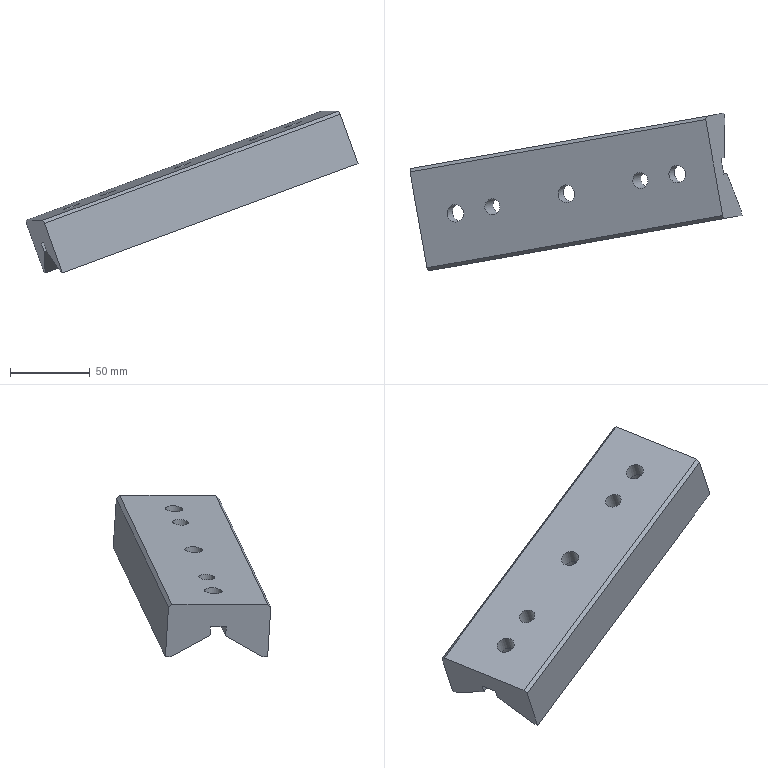Part | NX | features solid 2 | 1 solid | 36 faces | box 207.812 x 98.608 x 101.293 mm | volume 334850 mm3 | plane 28 | cylinder 8 | commonest cylinder face diameters 11 x3 17.5 x3 10 x2
STEP:
#1=CARTESIAN_POINT('',(1039.266,104.665,-184.286));
#2=VERTEX_POINT('',#1);
#3=CARTESIAN_POINT('',(1041.003,94.817,-184.286));
#4=VERTEX_POINT('',#3);
#5=CARTESIAN_POINT('',(1040.138,99.742,-184.285));
#6=DIRECTION('',(-0.3368,-0.05939,0.9397));
#7=DIRECTION('',(-0.9254,-0.1632,-0.342));
#8=AXIS2_PLACEMENT_3D('',#5,#6,#7);
#9=CIRCLE('',#8,5.);
#10=EDGE_CURVE('',#2,#4,#9,.T.);
#11=ORIENTED_EDGE('',*,*,#10,.T.);
#12=CARTESIAN_POINT('',(1001.381,87.831,-198.93));
#13=VERTEX_POINT('',#12);
#14=CARTESIAN_POINT('',(902.194,70.341,-235.588));
#15=DIRECTION('',(0.9254,0.1632,0.342));
#16=VECTOR('',#15,1000.);
#17=LINE('',#14,#16);
#18=EDGE_CURVE('',#13,#4,#17,.T.);
#19=ORIENTED_EDGE('',*,*,#18,.F.);
#20=CARTESIAN_POINT('',(999.644,97.679,-198.93));
#21=VERTEX_POINT('',#20);
#22=CARTESIAN_POINT('',(993.867,91.583,-201.386));
#23=DIRECTION('',(-0.3368,-0.05939,0.9397));
#24=DIRECTION('',(-0.9254,-0.1632,-0.342));
#25=AXIS2_PLACEMENT_3D('',#22,#23,#24);
#26=CIRCLE('',#25,8.75);
#27=EDGE_CURVE('',#13,#21,#26,.T.);
#28=ORIENTED_EDGE('',*,*,#27,.T.);
#29=CARTESIAN_POINT('',(900.458,80.189,-235.588));
#30=DIRECTION('',(0.9254,0.1632,0.342));
#31=VECTOR('',#30,1000.);
#32=LINE('',#29,#31);
#33=EDGE_CURVE('',#21,#2,#32,.T.);
#34=ORIENTED_EDGE('',*,*,#33,.T.);
#35=EDGE_LOOP('',(#11,#19,#28,#34));
#36=FACE_BOUND('',#35,.T.);
#37=CARTESIAN_POINT('',(900.458,80.189,-235.588));
#38=DIRECTION('',(-0.3368,-0.05939,0.9397));
#39=DIRECTION('',(-0.9254,-0.1632,-0.342));
#40=AXIS2_PLACEMENT_3D('',#37,#38,#39);
#41=PLANE('',#40);
#42=ADVANCED_FACE('',(#36),#41,.F.);
#43=CARTESIAN_POINT('',(1039.713,99.667,-168.479));
#44=VERTEX_POINT('',#43);
#45=CARTESIAN_POINT('',(1035.086,98.851,-170.19));
#46=DIRECTION('',(0.3368,0.05939,-0.9397));
#47=DIRECTION('',(0.9254,0.1632,0.342));
#48=AXIS2_PLACEMENT_3D('',#45,#46,#47);
#49=CIRCLE('',#48,5.);
#50=EDGE_CURVE('',#44,#44,#49,.T.);
#51=ORIENTED_EDGE('',*,*,#50,.T.);
#52=EDGE_LOOP('',(#51));
#53=FACE_BOUND('',#52,.T.);
#54=CARTESIAN_POINT('',(983.725,89.795,-189.172));
#55=VERTEX_POINT('',#54);
#56=CARTESIAN_POINT('',(988.815,90.692,-187.291));
#57=DIRECTION('',(0.3368,0.05939,-0.9397));
#58=DIRECTION('',(-0.9254,-0.1632,-0.342));
#59=AXIS2_PLACEMENT_3D('',#56,#57,#58);
#60=CIRCLE('',#59,5.5);
#61=EDGE_CURVE('',#55,#55,#60,.T.);
#62=ORIENTED_EDGE('',*,*,#61,.T.);
#63=EDGE_LOOP('',(#62));
#64=FACE_BOUND('',#63,.T.);
#65=CARTESIAN_POINT('',(947.171,83.349,-202.681));
#66=VERTEX_POINT('',#65);
#67=CARTESIAN_POINT('',(942.544,82.533,-204.392));
#68=DIRECTION('',(0.3368,0.05939,-0.9397));
#69=DIRECTION('',(0.9254,0.1632,0.342));
#70=AXIS2_PLACEMENT_3D('',#67,#68,#69);
#71=CIRCLE('',#70,5.);
#72=EDGE_CURVE('',#66,#66,#71,.T.);
#73=ORIENTED_EDGE('',*,*,#72,.T.);
#74=EDGE_LOOP('',(#73));
#75=FACE_BOUND('',#74,.T.);
#76=CARTESIAN_POINT('',(924.499,79.351,-211.061));
#77=VERTEX_POINT('',#76);
#78=CARTESIAN_POINT('',(919.409,78.454,-212.942));
#79=DIRECTION('',(0.3368,0.05939,-0.9397));
#80=DIRECTION('',(0.9254,0.1632,0.342));
#81=AXIS2_PLACEMENT_3D('',#78,#79,#80);
#82=CIRCLE('',#81,5.5);
#83=EDGE_CURVE('',#77,#77,#82,.T.);
#84=ORIENTED_EDGE('',*,*,#83,.T.);
#85=EDGE_LOOP('',(#84));
#86=FACE_BOUND('',#85,.T.);
#87=CARTESIAN_POINT('',(1063.311,103.828,-159.758));
#88=VERTEX_POINT('',#87);
#89=CARTESIAN_POINT('',(1058.221,102.93,-161.639));
#90=DIRECTION('',(0.3368,0.05939,-0.9397));
#91=DIRECTION('',(0.9254,0.1632,0.342));
#92=AXIS2_PLACEMENT_3D('',#89,#90,#91);
#93=CIRCLE('',#92,5.5);
#94=EDGE_CURVE('',#88,#88,#93,.T.);
#95=ORIENTED_EDGE('',*,*,#94,.T.);
#96=EDGE_LOOP('',(#95));
#97=FACE_BOUND('',#96,.T.);
#98=CARTESIAN_POINT('',(890.977,104.411,-221.493));
#99=VERTEX_POINT('',#98);
#100=CARTESIAN_POINT('',(901.57,44.338,-221.493));
#101=VERTEX_POINT('',#100);
#102=CARTESIAN_POINT('',(890.63,106.381,-221.493));
#103=DIRECTION('',(0.1736,-0.9848,0.));
#104=VECTOR('',#103,1000.);
#105=LINE('',#102,#104);
#106=EDGE_CURVE('',#99,#101,#105,.T.);
#107=ORIENTED_EDGE('',*,*,#106,.T.);
#108=CARTESIAN_POINT('',(1086.653,76.973,-153.089));
#109=VERTEX_POINT('',#108);
#110=CARTESIAN_POINT('',(901.57,44.338,-221.493));
#111=DIRECTION('',(0.9254,0.1632,0.342));
#112=VECTOR('',#111,1000.);
#113=LINE('',#110,#112);
#114=EDGE_CURVE('',#101,#109,#113,.T.);
#115=ORIENTED_EDGE('',*,*,#114,.T.);
#116=CARTESIAN_POINT('',(1076.06,137.046,-153.089));
#117=VERTEX_POINT('',#116);
#118=CARTESIAN_POINT('',(1075.713,139.016,-153.089));
#119=DIRECTION('',(0.1736,-0.9848,0.));
#120=VECTOR('',#119,1000.);
#121=LINE('',#118,#120);
#122=EDGE_CURVE('',#117,#109,#121,.T.);
#123=ORIENTED_EDGE('',*,*,#122,.F.);
#124=CARTESIAN_POINT('',(890.977,104.411,-221.493));
#125=DIRECTION('',(0.9254,0.1632,0.342));
#126=VECTOR('',#125,1000.);
#127=LINE('',#124,#126);
#128=EDGE_CURVE('',#99,#117,#127,.T.);
#129=ORIENTED_EDGE('',*,*,#128,.F.);
#130=EDGE_LOOP('',(#107,#115,#123,#129));
#131=FACE_BOUND('',#130,.T.);
#132=CARTESIAN_POINT('',(890.63,106.381,-221.493));
#133=DIRECTION('',(-0.3368,-0.05939,0.9397));
#134=DIRECTION('',(-0.9254,-0.1632,-0.342));
#135=AXIS2_PLACEMENT_3D('',#132,#133,#134);
#136=PLANE('',#135);
#137=ADVANCED_FACE('',(#53,#64,#75,#86,#97,#131),#136,.T.);
#138=CARTESIAN_POINT('',(946.728,88.348,-218.487));
#139=VERTEX_POINT('',#138);
#140=CARTESIAN_POINT('',(948.465,78.5,-218.487));
#141=VERTEX_POINT('',#140);
#142=CARTESIAN_POINT('',(947.597,83.424,-218.487));
#143=DIRECTION('',(-0.3368,-0.05939,0.9397));
#144=DIRECTION('',(-0.9254,-0.1632,-0.342));
#145=AXIS2_PLACEMENT_3D('',#142,#143,#144);
#146=CIRCLE('',#145,5.);
#147=EDGE_CURVE('',#139,#141,#146,.T.);
#148=ORIENTED_EDGE('',*,*,#147,.T.);
#149=CARTESIAN_POINT('',(931.975,75.592,-224.581));
#150=VERTEX_POINT('',#149);
#151=CARTESIAN_POINT('',(902.194,70.341,-235.588));
#152=DIRECTION('',(0.9254,0.1632,0.342));
#153=VECTOR('',#152,1000.);
#154=LINE('',#151,#153);
#155=EDGE_CURVE('',#150,#141,#154,.T.);
#156=ORIENTED_EDGE('',*,*,#155,.F.);
#157=CARTESIAN_POINT('',(930.238,85.44,-224.581));
#158=VERTEX_POINT('',#157);
#159=CARTESIAN_POINT('',(924.461,79.345,-227.037));
#160=DIRECTION('',(-0.3368,-0.05939,0.9397));
#161=DIRECTION('',(-0.9254,-0.1632,-0.342));
#162=AXIS2_PLACEMENT_3D('',#159,#160,#161);
#163=CIRCLE('',#162,8.75);
#164=EDGE_CURVE('',#150,#158,#163,.T.);
#165=ORIENTED_EDGE('',*,*,#164,.T.);
#166=CARTESIAN_POINT('',(900.458,80.189,-235.588));
#167=DIRECTION('',(0.9254,0.1632,0.342));
#168=VECTOR('',#167,1000.);
#169=LINE('',#166,#168);
#170=EDGE_CURVE('',#158,#139,#169,.T.);
#171=ORIENTED_EDGE('',*,*,#170,.T.);
#172=EDGE_LOOP('',(#148,#156,#165,#171));
#173=FACE_BOUND('',#172,.T.);
#174=CARTESIAN_POINT('',(900.458,80.189,-235.588));
#175=DIRECTION('',(-0.3368,-0.05939,0.9397));
#176=DIRECTION('',(-0.9254,-0.1632,-0.342));
#177=AXIS2_PLACEMENT_3D('',#174,#175,#176);
#178=PLANE('',#177);
#179=ADVANCED_FACE('',(#173),#178,.F.);
#180=CARTESIAN_POINT('',(986.354,95.335,-203.842));
#181=VERTEX_POINT('',#180);
#182=CARTESIAN_POINT('',(988.091,85.487,-203.842));
#183=VERTEX_POINT('',#182);
#184=CARTESIAN_POINT('',(993.867,91.583,-201.386));
#185=DIRECTION('',(-0.3368,-0.05939,0.9397));
#186=DIRECTION('',(-0.9254,-0.1632,-0.342));
#187=AXIS2_PLACEMENT_3D('',#184,#185,#186);
#188=CIRCLE('',#187,8.75);
#189=EDGE_CURVE('',#181,#183,#188,.T.);
#190=ORIENTED_EDGE('',*,*,#189,.T.);
#191=CARTESIAN_POINT('',(902.194,70.341,-235.588));
#192=DIRECTION('',(0.9254,0.1632,0.342));
#193=VECTOR('',#192,1000.);
#194=LINE('',#191,#193);
#195=EDGE_CURVE('',#141,#183,#194,.T.);
#196=ORIENTED_EDGE('',*,*,#195,.F.);
#197=CARTESIAN_POINT('',(947.597,83.424,-218.487));
#198=DIRECTION('',(-0.3368,-0.05939,0.9397));
#199=DIRECTION('',(-0.9254,-0.1632,-0.342));
#200=AXIS2_PLACEMENT_3D('',#197,#198,#199);
#201=CIRCLE('',#200,5.);
#202=EDGE_CURVE('',#141,#139,#201,.T.);
#203=ORIENTED_EDGE('',*,*,#202,.T.);
#204=CARTESIAN_POINT('',(900.458,80.189,-235.588));
#205=DIRECTION('',(0.9254,0.1632,0.342));
#206=VECTOR('',#205,1000.);
#207=LINE('',#204,#206);
#208=EDGE_CURVE('',#139,#181,#207,.T.);
#209=ORIENTED_EDGE('',*,*,#208,.T.);
#210=EDGE_LOOP('',(#190,#196,#203,#209));
#211=FACE_BOUND('',#210,.T.);
#212=CARTESIAN_POINT('',(900.458,80.189,-235.588));
#213=DIRECTION('',(-0.3368,-0.05939,0.9397));
#214=DIRECTION('',(-0.9254,-0.1632,-0.342));
#215=AXIS2_PLACEMENT_3D('',#212,#213,#214);
#216=PLANE('',#215);
#217=ADVANCED_FACE('',(#211),#216,.F.);
#218=CARTESIAN_POINT('',(1055.76,107.573,-178.19));
#219=VERTEX_POINT('',#218);
#220=CARTESIAN_POINT('',(1057.497,97.725,-178.19));
#221=VERTEX_POINT('',#220);
#222=CARTESIAN_POINT('',(1063.274,103.821,-175.734));
#223=DIRECTION('',(-0.3368,-0.05939,0.9397));
#224=DIRECTION('',(-0.9254,-0.1632,-0.342));
#225=AXIS2_PLACEMENT_3D('',#222,#223,#224);
#226=CIRCLE('',#225,8.75);
#227=EDGE_CURVE('',#219,#221,#226,.T.);
#228=ORIENTED_EDGE('',*,*,#227,.T.);
#229=CARTESIAN_POINT('',(902.194,70.341,-235.588));
#230=DIRECTION('',(0.9254,0.1632,0.342));
#231=VECTOR('',#230,1000.);
#232=LINE('',#229,#231);
#233=EDGE_CURVE('',#4,#221,#232,.T.);
#234=ORIENTED_EDGE('',*,*,#233,.F.);
#235=CARTESIAN_POINT('',(1040.138,99.742,-184.285));
#236=DIRECTION('',(-0.3368,-0.05939,0.9397));
#237=DIRECTION('',(-0.9254,-0.1632,-0.342));
#238=AXIS2_PLACEMENT_3D('',#235,#236,#237);
#239=CIRCLE('',#238,5.);
#240=EDGE_CURVE('',#4,#2,#239,.T.);
#241=ORIENTED_EDGE('',*,*,#240,.T.);
#242=CARTESIAN_POINT('',(900.458,80.189,-235.588));
#243=DIRECTION('',(0.9254,0.1632,0.342));
#244=VECTOR('',#243,1000.);
#245=LINE('',#242,#244);
#246=EDGE_CURVE('',#2,#219,#245,.T.);
#247=ORIENTED_EDGE('',*,*,#246,.T.);
#248=EDGE_LOOP('',(#228,#234,#241,#247));
#249=FACE_BOUND('',#248,.T.);
#250=CARTESIAN_POINT('',(900.458,80.189,-235.588));
#251=DIRECTION('',(-0.3368,-0.05939,0.9397));
#252=DIRECTION('',(-0.9254,-0.1632,-0.342));
#253=AXIS2_PLACEMENT_3D('',#250,#251,#252);
#254=PLANE('',#253);
#255=ADVANCED_FACE('',(#249),#254,.F.);
#256=CARTESIAN_POINT('',(1085.541,112.825,-167.184));
#257=VERTEX_POINT('',#256);
#258=CARTESIAN_POINT('',(1087.277,102.976,-167.184));
#259=VERTEX_POINT('',#258);
#260=CARTESIAN_POINT('',(1085.541,112.825,-167.184));
#261=DIRECTION('',(0.1736,-0.9848,0.));
#262=VECTOR('',#261,1000.);
#263=LINE('',#260,#262);
#264=EDGE_CURVE('',#257,#259,#263,.T.);
#265=ORIENTED_EDGE('',*,*,#264,.T.);
#266=CARTESIAN_POINT('',(1070.787,100.069,-173.278));
#267=VERTEX_POINT('',#266);
#268=CARTESIAN_POINT('',(902.194,70.341,-235.588));
#269=DIRECTION('',(0.9254,0.1632,0.342));
#270=VECTOR('',#269,1000.);
#271=LINE('',#268,#270);
#272=EDGE_CURVE('',#267,#259,#271,.T.);
#273=ORIENTED_EDGE('',*,*,#272,.F.);
#274=CARTESIAN_POINT('',(1069.051,109.917,-173.278));
#275=VERTEX_POINT('',#274);
#276=CARTESIAN_POINT('',(1063.274,103.821,-175.734));
#277=DIRECTION('',(-0.3368,-0.05939,0.9397));
#278=DIRECTION('',(-0.9254,-0.1632,-0.342));
#279=AXIS2_PLACEMENT_3D('',#276,#277,#278);
#280=CIRCLE('',#279,8.75);
#281=EDGE_CURVE('',#267,#275,#280,.T.);
#282=ORIENTED_EDGE('',*,*,#281,.T.);
#283=CARTESIAN_POINT('',(900.458,80.189,-235.588));
#284=DIRECTION('',(0.9254,0.1632,0.342));
#285=VECTOR('',#284,1000.);
#286=LINE('',#283,#285);
#287=EDGE_CURVE('',#275,#257,#286,.T.);
#288=ORIENTED_EDGE('',*,*,#287,.T.);
#289=EDGE_LOOP('',(#265,#273,#282,#288));
#290=FACE_BOUND('',#289,.T.);
#291=CARTESIAN_POINT('',(900.458,80.189,-235.588));
#292=DIRECTION('',(-0.3368,-0.05939,0.9397));
#293=DIRECTION('',(-0.9254,-0.1632,-0.342));
#294=AXIS2_PLACEMENT_3D('',#291,#292,#293);
#295=PLANE('',#294);
#296=ADVANCED_FACE('',(#290),#295,.F.);
#297=CARTESIAN_POINT('',(916.948,83.097,-229.493));
#298=VERTEX_POINT('',#297);
#299=CARTESIAN_POINT('',(918.684,73.249,-229.493));
#300=VERTEX_POINT('',#299);
#301=CARTESIAN_POINT('',(924.461,79.345,-227.037));
#302=DIRECTION('',(-0.3368,-0.05939,0.9397));
#303=DIRECTION('',(-0.9254,-0.1632,-0.342));
#304=AXIS2_PLACEMENT_3D('',#301,#302,#303);
#305=CIRCLE('',#304,8.75);
#306=EDGE_CURVE('',#298,#300,#305,.T.);
#307=ORIENTED_EDGE('',*,*,#306,.T.);
#308=CARTESIAN_POINT('',(902.194,70.341,-235.588));
#309=VERTEX_POINT('',#308);
#310=CARTESIAN_POINT('',(902.194,70.341,-235.588));
#311=DIRECTION('',(0.9254,0.1632,0.342));
#312=VECTOR('',#311,1000.);
#313=LINE('',#310,#312);
#314=EDGE_CURVE('',#309,#300,#313,.T.);
#315=ORIENTED_EDGE('',*,*,#314,.F.);
#316=CARTESIAN_POINT('',(900.458,80.189,-235.588));
#317=VERTEX_POINT('',#316);
#318=CARTESIAN_POINT('',(900.458,80.189,-235.588));
#319=DIRECTION('',(0.1736,-0.9848,0.));
#320=VECTOR('',#319,1000.);
#321=LINE('',#318,#320);
#322=EDGE_CURVE('',#317,#309,#321,.T.);
#323=ORIENTED_EDGE('',*,*,#322,.F.);
#324=CARTESIAN_POINT('',(900.458,80.189,-235.588));
#325=DIRECTION('',(0.9254,0.1632,0.342));
#326=VECTOR('',#325,1000.);
#327=LINE('',#324,#326);
#328=EDGE_CURVE('',#317,#298,#327,.T.);
#329=ORIENTED_EDGE('',*,*,#328,.T.);
#330=EDGE_LOOP('',(#307,#315,#323,#329));
#331=FACE_BOUND('',#330,.T.);
#332=CARTESIAN_POINT('',(900.458,80.189,-235.588));
#333=DIRECTION('',(-0.3368,-0.05939,0.9397));
#334=DIRECTION('',(-0.9254,-0.1632,-0.342));
#335=AXIS2_PLACEMENT_3D('',#332,#333,#334);
#336=PLANE('',#335);
#337=ADVANCED_FACE('',(#331),#336,.F.);
#338=ORIENTED_EDGE('',*,*,#322,.T.);
#339=CARTESIAN_POINT('',(904.177,70.691,-241.12));
#340=VERTEX_POINT('',#339);
#341=CARTESIAN_POINT('',(902.194,70.341,-235.588));
#342=DIRECTION('',(0.3368,0.05939,-0.9397));
#343=VECTOR('',#342,1000.);
#344=LINE('',#341,#343);
#345=EDGE_CURVE('',#309,#340,#344,.T.);
#346=ORIENTED_EDGE('',*,*,#345,.T.);
#347=CARTESIAN_POINT('',(913.175,47.456,-254.382));
#348=VERTEX_POINT('',#347);
#349=CARTESIAN_POINT('',(904.177,70.691,-241.12));
#350=DIRECTION('',(0.3188,-0.8232,-0.4698));
#351=VECTOR('',#350,1000.);
#352=LINE('',#349,#351);
#353=EDGE_CURVE('',#340,#348,#352,.T.);
#354=ORIENTED_EDGE('',*,*,#353,.T.);
#355=CARTESIAN_POINT('',(913.706,44.447,-254.382));
#356=VERTEX_POINT('',#355);
#357=CARTESIAN_POINT('',(913.706,44.447,-254.382));
#358=DIRECTION('',(-0.1736,0.9848,0.));
#359=VECTOR('',#358,1000.);
#360=LINE('',#357,#359);
#361=EDGE_CURVE('',#356,#348,#360,.T.);
#362=ORIENTED_EDGE('',*,*,#361,.F.);
#363=CARTESIAN_POINT('',(902.591,42.487,-223.372));
#364=VERTEX_POINT('',#363);
#365=CARTESIAN_POINT('',(901.917,42.368,-221.493));
#366=DIRECTION('',(0.3368,0.05939,-0.9397));
#367=VECTOR('',#366,1000.);
#368=LINE('',#365,#367);
#369=EDGE_CURVE('',#364,#356,#368,.T.);
#370=ORIENTED_EDGE('',*,*,#369,.F.);
#371=CARTESIAN_POINT('',(892.509,60.764,-204.813));
#372=DIRECTION('',(0.361,-0.6544,-0.6645));
#373=VECTOR('',#372,1000.);
#374=LINE('',#371,#373);
#375=EDGE_CURVE('',#364,#101,#374,.F.);
#376=ORIENTED_EDGE('',*,*,#375,.T.);
#377=ORIENTED_EDGE('',*,*,#106,.F.);
#378=CARTESIAN_POINT('',(891.304,106.499,-223.372));
#379=VERTEX_POINT('',#378);
#380=CARTESIAN_POINT('',(888.081,85.877,-204.813));
#381=DIRECTION('',(0.1154,0.7384,-0.6645));
#382=VECTOR('',#381,1000.);
#383=LINE('',#380,#382);
#384=EDGE_CURVE('',#379,#99,#383,.F.);
#385=ORIENTED_EDGE('',*,*,#384,.F.);
#386=CARTESIAN_POINT('',(902.419,108.459,-254.382));
#387=VERTEX_POINT('',#386);
#388=CARTESIAN_POINT('',(890.63,106.381,-221.493));
#389=DIRECTION('',(0.3368,0.05939,-0.9397));
#390=VECTOR('',#389,1000.);
#391=LINE('',#388,#390);
#392=EDGE_CURVE('',#379,#387,#391,.T.);
#393=ORIENTED_EDGE('',*,*,#392,.T.);
#394=CARTESIAN_POINT('',(902.949,105.451,-254.382));
#395=VERTEX_POINT('',#394);
#396=CARTESIAN_POINT('',(902.419,108.459,-254.382));
#397=DIRECTION('',(0.1736,-0.9848,0.));
#398=VECTOR('',#397,1000.);
#399=LINE('',#396,#398);
#400=EDGE_CURVE('',#387,#395,#399,.T.);
#401=ORIENTED_EDGE('',*,*,#400,.T.);
#402=CARTESIAN_POINT('',(902.44,80.539,-241.12));
#403=VERTEX_POINT('',#402);
#404=CARTESIAN_POINT('',(902.44,80.539,-241.12));
#405=DIRECTION('',(0.01803,0.8826,-0.4698));
#406=VECTOR('',#405,1000.);
#407=LINE('',#404,#406);
#408=EDGE_CURVE('',#403,#395,#407,.T.);
#409=ORIENTED_EDGE('',*,*,#408,.F.);
#410=CARTESIAN_POINT('',(900.458,80.189,-235.588));
#411=DIRECTION('',(0.3368,0.05939,-0.9397));
#412=VECTOR('',#411,1000.);
#413=LINE('',#410,#412);
#414=EDGE_CURVE('',#317,#403,#413,.T.);
#415=ORIENTED_EDGE('',*,*,#414,.F.);
#416=EDGE_LOOP('',(#338,#346,#354,#362,#370,#376,#377,#385,#393,#401,#409,#415));
#417=FACE_BOUND('',#416,.T.);
#418=CARTESIAN_POINT('',(895.405,79.298,-221.493));
#419=DIRECTION('',(-0.9254,-0.1632,-0.342));
#420=DIRECTION('',(0.3368,0.05939,-0.9397));
#421=AXIS2_PLACEMENT_3D('',#418,#419,#420);
#422=PLANE('',#421);
#423=ADVANCED_FACE('',(#417),#422,.T.);
#424=ORIENTED_EDGE('',*,*,#122,.T.);
#425=CARTESIAN_POINT('',(1087.674,75.122,-154.968));
#426=VERTEX_POINT('',#425);
#427=CARTESIAN_POINT('',(1086.653,76.973,-153.089));
#428=DIRECTION('',(-0.361,0.6544,0.6645));
#429=VECTOR('',#428,1000.);
#430=LINE('',#427,#429);
#431=EDGE_CURVE('',#109,#426,#430,.F.);
#432=ORIENTED_EDGE('',*,*,#431,.T.);
#433=CARTESIAN_POINT('',(1098.789,77.082,-185.978));
#434=VERTEX_POINT('',#433);
#435=CARTESIAN_POINT('',(1087.,75.003,-153.089));
#436=DIRECTION('',(0.3368,0.05939,-0.9397));
#437=VECTOR('',#436,1000.);
#438=LINE('',#435,#437);
#439=EDGE_CURVE('',#426,#434,#438,.T.);
#440=ORIENTED_EDGE('',*,*,#439,.T.);
#441=CARTESIAN_POINT('',(1098.259,80.091,-185.978));
#442=VERTEX_POINT('',#441);
#443=CARTESIAN_POINT('',(1098.789,77.082,-185.978));
#444=DIRECTION('',(-0.1736,0.9848,0.));
#445=VECTOR('',#444,1000.);
#446=LINE('',#443,#445);
#447=EDGE_CURVE('',#434,#442,#446,.T.);
#448=ORIENTED_EDGE('',*,*,#447,.T.);
#449=CARTESIAN_POINT('',(1089.26,103.326,-172.716));
#450=VERTEX_POINT('',#449);
#451=CARTESIAN_POINT('',(1089.26,103.326,-172.716));
#452=DIRECTION('',(0.3188,-0.8232,-0.4698));
#453=VECTOR('',#452,1000.);
#454=LINE('',#451,#453);
#455=EDGE_CURVE('',#450,#442,#454,.T.);
#456=ORIENTED_EDGE('',*,*,#455,.F.);
#457=CARTESIAN_POINT('',(1087.277,102.976,-167.184));
#458=DIRECTION('',(0.3368,0.05939,-0.9397));
#459=VECTOR('',#458,1000.);
#460=LINE('',#457,#459);
#461=EDGE_CURVE('',#259,#450,#460,.T.);
#462=ORIENTED_EDGE('',*,*,#461,.F.);
#463=ORIENTED_EDGE('',*,*,#264,.F.);
#464=CARTESIAN_POINT('',(1087.524,113.174,-172.716));
#465=VERTEX_POINT('',#464);
#466=CARTESIAN_POINT('',(1085.541,112.825,-167.184));
#467=DIRECTION('',(0.3368,0.05939,-0.9397));
#468=VECTOR('',#467,1000.);
#469=LINE('',#466,#468);
#470=EDGE_CURVE('',#257,#465,#469,.T.);
#471=ORIENTED_EDGE('',*,*,#470,.T.);
#472=CARTESIAN_POINT('',(1088.033,138.086,-185.978));
#473=VERTEX_POINT('',#472);
#474=CARTESIAN_POINT('',(1087.524,113.174,-172.716));
#475=DIRECTION('',(0.01803,0.8826,-0.4698));
#476=VECTOR('',#475,1000.);
#477=LINE('',#474,#476);
#478=EDGE_CURVE('',#465,#473,#477,.T.);
#479=ORIENTED_EDGE('',*,*,#478,.T.);
#480=CARTESIAN_POINT('',(1087.502,141.095,-185.978));
#481=VERTEX_POINT('',#480);
#482=CARTESIAN_POINT('',(1087.502,141.095,-185.978));
#483=DIRECTION('',(0.1736,-0.9848,0.));
#484=VECTOR('',#483,1000.);
#485=LINE('',#482,#484);
#486=EDGE_CURVE('',#481,#473,#485,.T.);
#487=ORIENTED_EDGE('',*,*,#486,.F.);
#488=CARTESIAN_POINT('',(1076.387,139.135,-154.968));
#489=VERTEX_POINT('',#488);
#490=CARTESIAN_POINT('',(1075.713,139.016,-153.089));
#491=DIRECTION('',(0.3368,0.05939,-0.9397));
#492=VECTOR('',#491,1000.);
#493=LINE('',#490,#492);
#494=EDGE_CURVE('',#489,#481,#493,.T.);
#495=ORIENTED_EDGE('',*,*,#494,.F.);
#496=CARTESIAN_POINT('',(1076.06,137.046,-153.089));
#497=DIRECTION('',(-0.1154,-0.7384,0.6645));
#498=VECTOR('',#497,1000.);
#499=LINE('',#496,#498);
#500=EDGE_CURVE('',#117,#489,#499,.F.);
#501=ORIENTED_EDGE('',*,*,#500,.F.);
#502=EDGE_LOOP('',(#424,#432,#440,#448,#456,#462,#463,#471,#479,#487,#495,#501));
#503=FACE_BOUND('',#502,.T.);
#504=CARTESIAN_POINT('',(1080.489,111.934,-153.089));
#505=DIRECTION('',(-0.9254,-0.1632,-0.342));
#506=DIRECTION('',(0.3368,0.05939,-0.9397));
#507=AXIS2_PLACEMENT_3D('',#504,#505,#506);
#508=PLANE('',#507);
#509=ADVANCED_FACE('',(#503),#508,.F.);
#510=ORIENTED_EDGE('',*,*,#94,.F.);
#511=EDGE_LOOP('',(#510));
#512=FACE_BOUND('',#511,.T.);
#513=CARTESIAN_POINT('',(1066.767,103.524,-169.18));
#514=VERTEX_POINT('',#513);
#515=CARTESIAN_POINT('',(1061.59,103.524,-171.036));
#516=DIRECTION('',(-0.3368,-0.05939,0.9397));
#517=DIRECTION('',(0.9414,0.,0.3374));
#518=AXIS2_PLACEMENT_3D('',#515,#516,#517);
#519=CIRCLE('',#518,5.5);
#520=EDGE_CURVE('',#514,#514,#519,.F.);
#521=ORIENTED_EDGE('',*,*,#520,.T.);
#522=EDGE_LOOP('',(#521));
#523=FACE_BOUND('',#522,.T.);
#524=CARTESIAN_POINT('',(1058.221,102.93,-161.639));
#525=DIRECTION('',(0.3368,0.05939,-0.9397));
#526=DIRECTION('',(0.9254,0.1632,0.342));
#527=AXIS2_PLACEMENT_3D('',#524,#525,#526);
#528=CYLINDRICAL_SURFACE('',#527,5.5);
#529=ADVANCED_FACE('',(#512,#523),#528,.F.);
#530=CARTESIAN_POINT('',(1069.826,103.524,-168.084));
#531=VERTEX_POINT('',#530);
#532=CARTESIAN_POINT('',(1061.59,103.524,-171.036));
#533=DIRECTION('',(-0.3368,-0.05939,0.9397));
#534=DIRECTION('',(0.9414,0.,0.3374));
#535=AXIS2_PLACEMENT_3D('',#532,#533,#534);
#536=CIRCLE('',#535,8.75);
#537=EDGE_CURVE('',#531,#531,#536,.F.);
#538=ORIENTED_EDGE('',*,*,#537,.F.);
#539=EDGE_LOOP('',(#538));
#540=FACE_BOUND('',#539,.T.);
#541=CARTESIAN_POINT('',(1059.48,98.075,-183.722));
#542=VERTEX_POINT('',#541);
#543=CARTESIAN_POINT('',(1055.139,97.31,-171.612));
#544=DIRECTION('',(0.3368,0.05939,-0.9397));
#545=VECTOR('',#544,1000.);
#546=LINE('',#543,#545);
#547=EDGE_CURVE('',#221,#542,#546,.T.);
#548=ORIENTED_EDGE('',*,*,#547,.F.);
#549=ORIENTED_EDGE('',*,*,#227,.F.);
#550=CARTESIAN_POINT('',(1057.743,107.923,-183.722));
#551=VERTEX_POINT('',#550);
#552=CARTESIAN_POINT('',(1053.403,107.158,-171.612));
#553=DIRECTION('',(0.3368,0.05939,-0.9397));
#554=VECTOR('',#553,1000.);
#555=LINE('',#552,#554);
#556=EDGE_CURVE('',#219,#551,#555,.T.);
#557=ORIENTED_EDGE('',*,*,#556,.T.);
#558=CARTESIAN_POINT('',(1071.033,110.266,-178.81));
#559=VERTEX_POINT('',#558);
#560=CARTESIAN_POINT('',(1064.284,103.999,-178.553));
#561=DIRECTION('',(0.3785,-0.441,-0.8138));
#562=DIRECTION('',(0.01803,0.8826,-0.4698));
#563=AXIS2_PLACEMENT_3D('',#560,#561,#562);
#564=ELLIPSE('',#563,10.104,8.75);
#565=EDGE_CURVE('',#551,#559,#564,.T.);
#566=ORIENTED_EDGE('',*,*,#565,.T.);
#567=CARTESIAN_POINT('',(1066.693,109.501,-166.701));
#568=DIRECTION('',(0.3368,0.05939,-0.9397));
#569=VECTOR('',#568,1000.);
#570=LINE('',#567,#569);
#571=EDGE_CURVE('',#559,#275,#570,.F.);
#572=ORIENTED_EDGE('',*,*,#571,.T.);
#573=ORIENTED_EDGE('',*,*,#281,.F.);
#574=CARTESIAN_POINT('',(1072.77,100.418,-178.81));
#575=VERTEX_POINT('',#574);
#576=CARTESIAN_POINT('',(1068.429,99.653,-166.701));
#577=DIRECTION('',(0.3368,0.05939,-0.9397));
#578=VECTOR('',#577,1000.);
#579=LINE('',#576,#578);
#580=EDGE_CURVE('',#575,#267,#579,.F.);
#581=ORIENTED_EDGE('',*,*,#580,.F.);
#582=CARTESIAN_POINT('',(1064.284,103.999,-178.553));
#583=DIRECTION('',(-0.2049,-0.5438,0.8138));
#584=DIRECTION('',(0.3188,-0.8232,-0.4698));
#585=AXIS2_PLACEMENT_3D('',#582,#583,#584);
#586=ELLIPSE('',#585,10.104,8.75);
#587=EDGE_CURVE('',#542,#575,#586,.T.);
#588=ORIENTED_EDGE('',*,*,#587,.F.);
#589=EDGE_LOOP('',(#548,#549,#557,#566,#572,#573,#581,#588));
#590=FACE_BOUND('',#589,.T.);
#591=CARTESIAN_POINT('',(1060.916,103.405,-169.157));
#592=DIRECTION('',(0.3368,0.05939,-0.9397));
#593=DIRECTION('',(0.9254,0.1632,0.342));
#594=AXIS2_PLACEMENT_3D('',#591,#592,#593);
#595=CYLINDRICAL_SURFACE('',#594,8.75);
#596=ADVANCED_FACE('',(#540,#590),#595,.F.);
#597=ORIENTED_EDGE('',*,*,#520,.F.);
#598=EDGE_LOOP('',(#597));
#599=FACE_BOUND('',#598,.T.);
#600=ORIENTED_EDGE('',*,*,#537,.T.);
#601=EDGE_LOOP('',(#600));
#602=FACE_BOUND('',#601,.T.);
#603=CARTESIAN_POINT('',(1015.319,95.365,-188.137));
#604=DIRECTION('',(-0.3368,-0.05939,0.9397));
#605=DIRECTION('',(-0.9254,-0.1632,-0.342));
#606=AXIS2_PLACEMENT_3D('',#603,#604,#605);
#607=PLANE('',#606);
#608=ADVANCED_FACE('',(#599,#602),#607,.F.);
#609=ORIENTED_EDGE('',*,*,#50,.F.);
#610=EDGE_LOOP('',(#609));
#611=FACE_BOUND('',#610,.T.);
#612=ORIENTED_EDGE('',*,*,#240,.F.);
#613=ORIENTED_EDGE('',*,*,#10,.F.);
#614=EDGE_LOOP('',(#612,#613));
#615=FACE_BOUND('',#614,.T.);
#616=CARTESIAN_POINT('',(1035.086,98.851,-170.19));
#617=DIRECTION('',(0.3368,0.05939,-0.9397));
#618=DIRECTION('',(0.9254,0.1632,0.342));
#619=AXIS2_PLACEMENT_3D('',#616,#617,#618);
#620=CYLINDRICAL_SURFACE('',#619,5.);
#621=ADVANCED_FACE('',(#611,#615),#620,.F.);
#622=ORIENTED_EDGE('',*,*,#72,.F.);
#623=EDGE_LOOP('',(#622));
#624=FACE_BOUND('',#623,.T.);
#625=ORIENTED_EDGE('',*,*,#202,.F.);
#626=ORIENTED_EDGE('',*,*,#147,.F.);
#627=EDGE_LOOP('',(#625,#626));
#628=FACE_BOUND('',#627,.T.);
#629=CARTESIAN_POINT('',(942.544,82.533,-204.392));
#630=DIRECTION('',(0.3368,0.05939,-0.9397));
#631=DIRECTION('',(0.9254,0.1632,0.342));
#632=AXIS2_PLACEMENT_3D('',#629,#630,#631);
#633=CYLINDRICAL_SURFACE('',#632,5.);
#634=ADVANCED_FACE('',(#624,#628),#633,.F.);
#635=CARTESIAN_POINT('',(927.955,79.048,-220.483));
#636=VERTEX_POINT('',#635);
#637=CARTESIAN_POINT('',(922.777,79.048,-222.339));
#638=DIRECTION('',(-0.3368,-0.05939,0.9397));
#639=DIRECTION('',(0.9414,0.,0.3374));
#640=AXIS2_PLACEMENT_3D('',#637,#638,#639);
#641=CIRCLE('',#640,5.5);
#642=EDGE_CURVE('',#636,#636,#641,.F.);
#643=ORIENTED_EDGE('',*,*,#642,.T.);
#644=EDGE_LOOP('',(#643));
#645=FACE_BOUND('',#644,.T.);
#646=ORIENTED_EDGE('',*,*,#83,.F.);
#647=EDGE_LOOP('',(#646));
#648=FACE_BOUND('',#647,.T.);
#649=CARTESIAN_POINT('',(919.409,78.454,-212.942));
#650=DIRECTION('',(0.3368,0.05939,-0.9397));
#651=DIRECTION('',(0.9254,0.1632,0.342));
#652=AXIS2_PLACEMENT_3D('',#649,#650,#651);
#653=CYLINDRICAL_SURFACE('',#652,5.5);
#654=ADVANCED_FACE('',(#645,#648),#653,.F.);
#655=ORIENTED_EDGE('',*,*,#164,.F.);
#656=CARTESIAN_POINT('',(933.957,75.942,-230.113));
#657=VERTEX_POINT('',#656);
#658=CARTESIAN_POINT('',(929.617,75.177,-218.004));
#659=DIRECTION('',(0.3368,0.05939,-0.9397));
#660=VECTOR('',#659,1000.);
#661=LINE('',#658,#660);
#662=EDGE_CURVE('',#657,#150,#661,.F.);
#663=ORIENTED_EDGE('',*,*,#662,.F.);
#664=CARTESIAN_POINT('',(920.667,73.599,-235.025));
#665=VERTEX_POINT('',#664);
#666=CARTESIAN_POINT('',(925.472,79.523,-229.856));
#667=DIRECTION('',(-0.2049,-0.5438,0.8138));
#668=DIRECTION('',(0.3188,-0.8232,-0.4698));
#669=AXIS2_PLACEMENT_3D('',#666,#667,#668);
#670=ELLIPSE('',#669,10.104,8.75);
#671=EDGE_CURVE('',#665,#657,#670,.T.);
#672=ORIENTED_EDGE('',*,*,#671,.F.);
#673=CARTESIAN_POINT('',(916.327,72.833,-222.916));
#674=DIRECTION('',(0.3368,0.05939,-0.9397));
#675=VECTOR('',#674,1000.);
#676=LINE('',#673,#675);
#677=EDGE_CURVE('',#300,#665,#676,.T.);
#678=ORIENTED_EDGE('',*,*,#677,.F.);
#679=ORIENTED_EDGE('',*,*,#306,.F.);
#680=CARTESIAN_POINT('',(918.931,83.447,-235.025));
#681=VERTEX_POINT('',#680);
#682=CARTESIAN_POINT('',(914.59,82.681,-222.916));
#683=DIRECTION('',(0.3368,0.05939,-0.9397));
#684=VECTOR('',#683,1000.);
#685=LINE('',#682,#684);
#686=EDGE_CURVE('',#298,#681,#685,.T.);
#687=ORIENTED_EDGE('',*,*,#686,.T.);
#688=CARTESIAN_POINT('',(932.221,85.79,-230.113));
#689=VERTEX_POINT('',#688);
#690=CARTESIAN_POINT('',(925.472,79.523,-229.856));
#691=DIRECTION('',(0.3785,-0.441,-0.8138));
#692=DIRECTION('',(0.01803,0.8826,-0.4698));
#693=AXIS2_PLACEMENT_3D('',#690,#691,#692);
#694=ELLIPSE('',#693,10.104,8.75);
#695=EDGE_CURVE('',#681,#689,#694,.T.);
#696=ORIENTED_EDGE('',*,*,#695,.T.);
#697=CARTESIAN_POINT('',(927.88,85.025,-218.004));
#698=DIRECTION('',(0.3368,0.05939,-0.9397));
#699=VECTOR('',#698,1000.);
#700=LINE('',#697,#699);
#701=EDGE_CURVE('',#689,#158,#700,.F.);
#702=ORIENTED_EDGE('',*,*,#701,.T.);
#703=EDGE_LOOP('',(#655,#663,#672,#678,#679,#687,#696,#702));
#704=FACE_BOUND('',#703,.T.);
#705=CARTESIAN_POINT('',(931.014,79.048,-219.387));
#706=VERTEX_POINT('',#705);
#707=CARTESIAN_POINT('',(922.777,79.048,-222.339));
#708=DIRECTION('',(-0.3368,-0.05939,0.9397));
#709=DIRECTION('',(0.9414,0.,0.3374));
#710=AXIS2_PLACEMENT_3D('',#707,#708,#709);
#711=CIRCLE('',#710,8.75);
#712=EDGE_CURVE('',#706,#706,#711,.F.);
#713=ORIENTED_EDGE('',*,*,#712,.F.);
#714=EDGE_LOOP('',(#713));
#715=FACE_BOUND('',#714,.T.);
#716=CARTESIAN_POINT('',(922.103,78.929,-220.46));
#717=DIRECTION('',(0.3368,0.05939,-0.9397));
#718=DIRECTION('',(0.9254,0.1632,0.342));
#719=AXIS2_PLACEMENT_3D('',#716,#717,#718);
#720=CYLINDRICAL_SURFACE('',#719,8.75);
#721=ADVANCED_FACE('',(#704,#715),#720,.F.);
#722=ORIENTED_EDGE('',*,*,#712,.T.);
#723=EDGE_LOOP('',(#722));
#724=FACE_BOUND('',#723,.T.);
#725=ORIENTED_EDGE('',*,*,#642,.F.);
#726=EDGE_LOOP('',(#725));
#727=FACE_BOUND('',#726,.T.);
#728=CARTESIAN_POINT('',(922.777,79.048,-222.339));
#729=DIRECTION('',(-0.3368,-0.05939,0.9397));
#730=DIRECTION('',(-0.9254,-0.1632,-0.342));
#731=AXIS2_PLACEMENT_3D('',#728,#729,#730);
#732=PLANE('',#731);
#733=ADVANCED_FACE('',(#724,#727),#732,.F.);
#734=ORIENTED_EDGE('',*,*,#27,.F.);
#735=CARTESIAN_POINT('',(1003.364,88.18,-204.462));
#736=VERTEX_POINT('',#735);
#737=CARTESIAN_POINT('',(999.023,87.415,-192.352));
#738=DIRECTION('',(0.3368,0.05939,-0.9397));
#739=VECTOR('',#738,1000.);
#740=LINE('',#737,#739);
#741=EDGE_CURVE('',#13,#736,#740,.T.);
#742=ORIENTED_EDGE('',*,*,#741,.T.);
#743=CARTESIAN_POINT('',(990.073,85.837,-209.374));
#744=VERTEX_POINT('',#743);
#745=CARTESIAN_POINT('',(994.878,91.761,-204.205));
#746=DIRECTION('',(0.2049,0.5438,-0.8138));
#747=DIRECTION('',(0.3188,-0.8232,-0.4698));
#748=AXIS2_PLACEMENT_3D('',#745,#746,#747);
#749=ELLIPSE('',#748,10.104,8.75);
#750=EDGE_CURVE('',#736,#744,#749,.T.);
#751=ORIENTED_EDGE('',*,*,#750,.T.);
#752=CARTESIAN_POINT('',(985.733,85.071,-197.264));
#753=DIRECTION('',(0.3368,0.05939,-0.9397));
#754=VECTOR('',#753,1000.);
#755=LINE('',#752,#754);
#756=EDGE_CURVE('',#744,#183,#755,.F.);
#757=ORIENTED_EDGE('',*,*,#756,.T.);
#758=ORIENTED_EDGE('',*,*,#189,.F.);
#759=CARTESIAN_POINT('',(988.337,95.685,-209.374));
#760=VERTEX_POINT('',#759);
#761=CARTESIAN_POINT('',(983.996,94.919,-197.264));
#762=DIRECTION('',(0.3368,0.05939,-0.9397));
#763=VECTOR('',#762,1000.);
#764=LINE('',#761,#763);
#765=EDGE_CURVE('',#760,#181,#764,.F.);
#766=ORIENTED_EDGE('',*,*,#765,.F.);
#767=CARTESIAN_POINT('',(1001.627,98.028,-204.462));
#768=VERTEX_POINT('',#767);
#769=CARTESIAN_POINT('',(994.878,91.761,-204.205));
#770=DIRECTION('',(-0.3785,0.441,0.8138));
#771=DIRECTION('',(0.01803,0.8826,-0.4698));
#772=AXIS2_PLACEMENT_3D('',#769,#770,#771);
#773=ELLIPSE('',#772,10.104,8.75);
#774=EDGE_CURVE('',#768,#760,#773,.T.);
#775=ORIENTED_EDGE('',*,*,#774,.F.);
#776=CARTESIAN_POINT('',(997.287,97.263,-192.352));
#777=DIRECTION('',(0.3368,0.05939,-0.9397));
#778=VECTOR('',#777,1000.);
#779=LINE('',#776,#778);
#780=EDGE_CURVE('',#21,#768,#779,.T.);
#781=ORIENTED_EDGE('',*,*,#780,.F.);
#782=EDGE_LOOP('',(#734,#742,#751,#757,#758,#766,#775,#781));
#783=FACE_BOUND('',#782,.T.);
#784=CARTESIAN_POINT('',(1000.42,91.286,-193.735));
#785=VERTEX_POINT('',#784);
#786=CARTESIAN_POINT('',(992.183,91.286,-196.687));
#787=DIRECTION('',(-0.3368,-0.05939,0.9397));
#788=DIRECTION('',(0.9414,0.,0.3374));
#789=AXIS2_PLACEMENT_3D('',#786,#787,#788);
#790=CIRCLE('',#789,8.75);
#791=EDGE_CURVE('',#785,#785,#790,.T.);
#792=ORIENTED_EDGE('',*,*,#791,.T.);
#793=EDGE_LOOP('',(#792));
#794=FACE_BOUND('',#793,.T.);
#795=CARTESIAN_POINT('',(991.51,91.167,-194.808));
#796=DIRECTION('',(0.3368,0.05939,-0.9397));
#797=DIRECTION('',(-0.9254,-0.1632,-0.342));
#798=AXIS2_PLACEMENT_3D('',#795,#796,#797);
#799=CYLINDRICAL_SURFACE('',#798,8.75);
#800=ADVANCED_FACE('',(#783,#794),#799,.F.);
#801=ORIENTED_EDGE('',*,*,#791,.F.);
#802=EDGE_LOOP('',(#801));
#803=FACE_BOUND('',#802,.T.);
#804=CARTESIAN_POINT('',(997.361,91.286,-194.832));
#805=VERTEX_POINT('',#804);
#806=CARTESIAN_POINT('',(992.183,91.286,-196.687));
#807=DIRECTION('',(-0.3368,-0.05939,0.9397));
#808=DIRECTION('',(0.9414,0.,0.3374));
#809=AXIS2_PLACEMENT_3D('',#806,#807,#808);
#810=CIRCLE('',#809,5.5);
#811=EDGE_CURVE('',#805,#805,#810,.T.);
#812=ORIENTED_EDGE('',*,*,#811,.T.);
#813=EDGE_LOOP('',(#812));
#814=FACE_BOUND('',#813,.T.);
#815=CARTESIAN_POINT('',(992.183,91.286,-196.687));
#816=DIRECTION('',(-0.3368,-0.05939,0.9397));
#817=DIRECTION('',(0.9254,0.1632,0.342));
#818=AXIS2_PLACEMENT_3D('',#815,#816,#817);
#819=PLANE('',#818);
#820=ADVANCED_FACE('',(#803,#814),#819,.F.);
#821=ORIENTED_EDGE('',*,*,#61,.F.);
#822=EDGE_LOOP('',(#821));
#823=FACE_BOUND('',#822,.T.);
#824=ORIENTED_EDGE('',*,*,#811,.F.);
#825=EDGE_LOOP('',(#824));
#826=FACE_BOUND('',#825,.T.);
#827=CARTESIAN_POINT('',(988.815,90.692,-187.291));
#828=DIRECTION('',(0.3368,0.05939,-0.9397));
#829=DIRECTION('',(-0.9254,-0.1632,-0.342));
#830=AXIS2_PLACEMENT_3D('',#827,#828,#829);
#831=CYLINDRICAL_SURFACE('',#830,5.5);
#832=ADVANCED_FACE('',(#823,#826),#831,.F.);
#833=ORIENTED_EDGE('',*,*,#33,.F.);
#834=ORIENTED_EDGE('',*,*,#780,.T.);
#835=CARTESIAN_POINT('',(902.44,80.539,-241.12));
#836=DIRECTION('',(0.9254,0.1632,0.342));
#837=VECTOR('',#836,1000.);
#838=LINE('',#835,#837);
#839=EDGE_CURVE('',#768,#551,#838,.T.);
#840=ORIENTED_EDGE('',*,*,#839,.T.);
#841=ORIENTED_EDGE('',*,*,#556,.F.);
#842=ORIENTED_EDGE('',*,*,#246,.F.);
#843=EDGE_LOOP('',(#833,#834,#840,#841,#842));
#844=FACE_BOUND('',#843,.T.);
#845=CARTESIAN_POINT('',(900.458,80.189,-235.588));
#846=DIRECTION('',(-0.1736,0.9848,0.));
#847=DIRECTION('',(-0.3368,-0.05939,0.9397));
#848=AXIS2_PLACEMENT_3D('',#845,#846,#847);
#849=PLANE('',#848);
#850=ADVANCED_FACE('',(#844),#849,.F.);
#851=ORIENTED_EDGE('',*,*,#328,.F.);
#852=ORIENTED_EDGE('',*,*,#414,.T.);
#853=CARTESIAN_POINT('',(902.44,80.539,-241.12));
#854=DIRECTION('',(0.9254,0.1632,0.342));
#855=VECTOR('',#854,1000.);
#856=LINE('',#853,#855);
#857=EDGE_CURVE('',#403,#681,#856,.T.);
#858=ORIENTED_EDGE('',*,*,#857,.T.);
#859=ORIENTED_EDGE('',*,*,#686,.F.);
#860=EDGE_LOOP('',(#851,#852,#858,#859));
#861=FACE_BOUND('',#860,.T.);
#862=CARTESIAN_POINT('',(900.458,80.189,-235.588));
#863=DIRECTION('',(-0.1736,0.9848,0.));
#864=DIRECTION('',(-0.3368,-0.05939,0.9397));
#865=AXIS2_PLACEMENT_3D('',#862,#863,#864);
#866=PLANE('',#865);
#867=ADVANCED_FACE('',(#861),#866,.F.);
#868=ORIENTED_EDGE('',*,*,#701,.F.);
#869=CARTESIAN_POINT('',(902.44,80.539,-241.12));
#870=DIRECTION('',(-0.9254,-0.1632,-0.342));
#871=VECTOR('',#870,1000.);
#872=LINE('',#869,#871);
#873=EDGE_CURVE('',#689,#760,#872,.F.);
#874=ORIENTED_EDGE('',*,*,#873,.T.);
#875=ORIENTED_EDGE('',*,*,#765,.T.);
#876=ORIENTED_EDGE('',*,*,#208,.F.);
#877=ORIENTED_EDGE('',*,*,#170,.F.);
#878=EDGE_LOOP('',(#868,#874,#875,#876,#877));
#879=FACE_BOUND('',#878,.T.);
#880=CARTESIAN_POINT('',(900.458,80.189,-235.588));
#881=DIRECTION('',(-0.1736,0.9848,0.));
#882=DIRECTION('',(-0.3368,-0.05939,0.9397));
#883=AXIS2_PLACEMENT_3D('',#880,#881,#882);
#884=PLANE('',#883);
#885=ADVANCED_FACE('',(#879),#884,.F.);
#886=ORIENTED_EDGE('',*,*,#494,.T.);
#887=CARTESIAN_POINT('',(902.419,108.459,-254.382));
#888=DIRECTION('',(0.9254,0.1632,0.342));
#889=VECTOR('',#888,1000.);
#890=LINE('',#887,#889);
#891=EDGE_CURVE('',#387,#481,#890,.T.);
#892=ORIENTED_EDGE('',*,*,#891,.F.);
#893=ORIENTED_EDGE('',*,*,#392,.F.);
#894=CARTESIAN_POINT('',(891.304,106.499,-223.372));
#895=DIRECTION('',(-0.9254,-0.1632,-0.342));
#896=VECTOR('',#895,1000.);
#897=LINE('',#894,#896);
#898=EDGE_CURVE('',#489,#379,#897,.T.);
#899=ORIENTED_EDGE('',*,*,#898,.F.);
#900=EDGE_LOOP('',(#886,#892,#893,#899));
#901=FACE_BOUND('',#900,.T.);
#902=CARTESIAN_POINT('',(890.63,106.381,-221.493));
#903=DIRECTION('',(-0.1736,0.9848,0.));
#904=DIRECTION('',(-0.3368,-0.05939,0.9397));
#905=AXIS2_PLACEMENT_3D('',#902,#903,#904);
#906=PLANE('',#905);
#907=ADVANCED_FACE('',(#901),#906,.T.);
#908=ORIENTED_EDGE('',*,*,#486,.T.);
#909=CARTESIAN_POINT('',(902.949,105.451,-254.382));
#910=DIRECTION('',(0.9254,0.1632,0.342));
#911=VECTOR('',#910,1000.);
#912=LINE('',#909,#911);
#913=EDGE_CURVE('',#395,#473,#912,.T.);
#914=ORIENTED_EDGE('',*,*,#913,.F.);
#915=ORIENTED_EDGE('',*,*,#400,.F.);
#916=ORIENTED_EDGE('',*,*,#891,.T.);
#917=EDGE_LOOP('',(#908,#914,#915,#916));
#918=FACE_BOUND('',#917,.T.);
#919=CARTESIAN_POINT('',(902.419,108.459,-254.382));
#920=DIRECTION('',(0.3368,0.05939,-0.9397));
#921=DIRECTION('',(0.9254,0.1632,0.342));
#922=AXIS2_PLACEMENT_3D('',#919,#920,#921);
#923=PLANE('',#922);
#924=ADVANCED_FACE('',(#918),#923,.T.);
#925=ORIENTED_EDGE('',*,*,#839,.F.);
#926=ORIENTED_EDGE('',*,*,#774,.T.);
#927=ORIENTED_EDGE('',*,*,#873,.F.);
#928=ORIENTED_EDGE('',*,*,#695,.F.);
#929=ORIENTED_EDGE('',*,*,#857,.F.);
#930=ORIENTED_EDGE('',*,*,#408,.T.);
#931=ORIENTED_EDGE('',*,*,#913,.T.);
#932=ORIENTED_EDGE('',*,*,#478,.F.);
#933=CARTESIAN_POINT('',(902.44,80.539,-241.12));
#934=DIRECTION('',(0.9254,0.1632,0.342));
#935=VECTOR('',#934,1000.);
#936=LINE('',#933,#935);
#937=EDGE_CURVE('',#559,#465,#936,.T.);
#938=ORIENTED_EDGE('',*,*,#937,.F.);
#939=ORIENTED_EDGE('',*,*,#565,.F.);
#940=EDGE_LOOP('',(#925,#926,#927,#928,#929,#930,#931,#932,#938,#939));
#941=FACE_BOUND('',#940,.T.);
#942=CARTESIAN_POINT('',(902.44,80.539,-241.12));
#943=DIRECTION('',(-0.3785,0.441,0.8138));
#944=DIRECTION('',(-0.01803,-0.8826,0.4698));
#945=AXIS2_PLACEMENT_3D('',#942,#943,#944);
#946=PLANE('',#945);
#947=ADVANCED_FACE('',(#941),#946,.F.);
#948=ORIENTED_EDGE('',*,*,#937,.T.);
#949=ORIENTED_EDGE('',*,*,#470,.F.);
#950=ORIENTED_EDGE('',*,*,#287,.F.);
#951=ORIENTED_EDGE('',*,*,#571,.F.);
#952=EDGE_LOOP('',(#948,#949,#950,#951));
#953=FACE_BOUND('',#952,.T.);
#954=CARTESIAN_POINT('',(900.458,80.189,-235.588));
#955=DIRECTION('',(-0.1736,0.9848,0.));
#956=DIRECTION('',(-0.3368,-0.05939,0.9397));
#957=AXIS2_PLACEMENT_3D('',#954,#955,#956);
#958=PLANE('',#957);
#959=ADVANCED_FACE('',(#953),#958,.F.);
#960=ORIENTED_EDGE('',*,*,#384,.T.);
#961=ORIENTED_EDGE('',*,*,#128,.T.);
#962=ORIENTED_EDGE('',*,*,#500,.T.);
#963=ORIENTED_EDGE('',*,*,#898,.T.);
#964=EDGE_LOOP('',(#960,#961,#962,#963));
#965=FACE_BOUND('',#964,.T.);
#966=CARTESIAN_POINT('',(890.977,104.411,-221.493));
#967=DIRECTION('',(0.361,-0.6544,-0.6645));
#968=DIRECTION('',(0.1154,0.7384,-0.6645));
#969=AXIS2_PLACEMENT_3D('',#966,#967,#968);
#970=PLANE('',#969);
#971=ADVANCED_FACE('',(#965),#970,.F.);
#972=ORIENTED_EDGE('',*,*,#18,.T.);
#973=ORIENTED_EDGE('',*,*,#233,.T.);
#974=ORIENTED_EDGE('',*,*,#547,.T.);
#975=CARTESIAN_POINT('',(904.177,70.691,-241.12));
#976=DIRECTION('',(0.9254,0.1632,0.342));
#977=VECTOR('',#976,1000.);
#978=LINE('',#975,#977);
#979=EDGE_CURVE('',#736,#542,#978,.T.);
#980=ORIENTED_EDGE('',*,*,#979,.F.);
#981=ORIENTED_EDGE('',*,*,#741,.F.);
#982=EDGE_LOOP('',(#972,#973,#974,#980,#981));
#983=FACE_BOUND('',#982,.T.);
#984=CARTESIAN_POINT('',(902.194,70.341,-235.588));
#985=DIRECTION('',(0.1736,-0.9848,0.));
#986=DIRECTION('',(-0.3368,-0.05939,0.9397));
#987=AXIS2_PLACEMENT_3D('',#984,#985,#986);
#988=PLANE('',#987);
#989=ADVANCED_FACE('',(#983),#988,.F.);
#990=ORIENTED_EDGE('',*,*,#314,.T.);
#991=ORIENTED_EDGE('',*,*,#677,.T.);
#992=CARTESIAN_POINT('',(904.177,70.691,-241.12));
#993=DIRECTION('',(0.9254,0.1632,0.342));
#994=VECTOR('',#993,1000.);
#995=LINE('',#992,#994);
#996=EDGE_CURVE('',#340,#665,#995,.T.);
#997=ORIENTED_EDGE('',*,*,#996,.F.);
#998=ORIENTED_EDGE('',*,*,#345,.F.);
#999=EDGE_LOOP('',(#990,#991,#997,#998));
#1000=FACE_BOUND('',#999,.T.);
#1001=CARTESIAN_POINT('',(902.194,70.341,-235.588));
#1002=DIRECTION('',(0.1736,-0.9848,0.));
#1003=DIRECTION('',(-0.3368,-0.05939,0.9397));
#1004=AXIS2_PLACEMENT_3D('',#1001,#1002,#1003);
#1005=PLANE('',#1004);
#1006=ADVANCED_FACE('',(#1000),#1005,.F.);
#1007=ORIENTED_EDGE('',*,*,#756,.F.);
#1008=CARTESIAN_POINT('',(904.177,70.691,-241.12));
#1009=DIRECTION('',(0.9254,0.1632,0.342));
#1010=VECTOR('',#1009,1000.);
#1011=LINE('',#1008,#1010);
#1012=EDGE_CURVE('',#657,#744,#1011,.T.);
#1013=ORIENTED_EDGE('',*,*,#1012,.F.);
#1014=ORIENTED_EDGE('',*,*,#662,.T.);
#1015=ORIENTED_EDGE('',*,*,#155,.T.);
#1016=ORIENTED_EDGE('',*,*,#195,.T.);
#1017=EDGE_LOOP('',(#1007,#1013,#1014,#1015,#1016));
#1018=FACE_BOUND('',#1017,.T.);
#1019=CARTESIAN_POINT('',(902.194,70.341,-235.588));
#1020=DIRECTION('',(0.1736,-0.9848,0.));
#1021=DIRECTION('',(-0.3368,-0.05939,0.9397));
#1022=AXIS2_PLACEMENT_3D('',#1019,#1020,#1021);
#1023=PLANE('',#1022);
#1024=ADVANCED_FACE('',(#1018),#1023,.F.);
#1025=ORIENTED_EDGE('',*,*,#439,.F.);
#1026=CARTESIAN_POINT('',(902.591,42.487,-223.372));
#1027=DIRECTION('',(-0.9254,-0.1632,-0.342));
#1028=VECTOR('',#1027,1000.);
#1029=LINE('',#1026,#1028);
#1030=EDGE_CURVE('',#426,#364,#1029,.T.);
#1031=ORIENTED_EDGE('',*,*,#1030,.T.);
#1032=ORIENTED_EDGE('',*,*,#369,.T.);
#1033=CARTESIAN_POINT('',(913.706,44.447,-254.382));
#1034=DIRECTION('',(0.9254,0.1632,0.342));
#1035=VECTOR('',#1034,1000.);
#1036=LINE('',#1033,#1035);
#1037=EDGE_CURVE('',#356,#434,#1036,.T.);
#1038=ORIENTED_EDGE('',*,*,#1037,.T.);
#1039=EDGE_LOOP('',(#1025,#1031,#1032,#1038));
#1040=FACE_BOUND('',#1039,.T.);
#1041=CARTESIAN_POINT('',(901.917,42.368,-221.493));
#1042=DIRECTION('',(0.1736,-0.9848,0.));
#1043=DIRECTION('',(-0.3368,-0.05939,0.9397));
#1044=AXIS2_PLACEMENT_3D('',#1041,#1042,#1043);
#1045=PLANE('',#1044);
#1046=ADVANCED_FACE('',(#1040),#1045,.T.);
#1047=ORIENTED_EDGE('',*,*,#447,.F.);
#1048=ORIENTED_EDGE('',*,*,#1037,.F.);
#1049=ORIENTED_EDGE('',*,*,#361,.T.);
#1050=CARTESIAN_POINT('',(913.175,47.456,-254.382));
#1051=DIRECTION('',(0.9254,0.1632,0.342));
#1052=VECTOR('',#1051,1000.);
#1053=LINE('',#1050,#1052);
#1054=EDGE_CURVE('',#348,#442,#1053,.T.);
#1055=ORIENTED_EDGE('',*,*,#1054,.T.);
#1056=EDGE_LOOP('',(#1047,#1048,#1049,#1055));
#1057=FACE_BOUND('',#1056,.T.);
#1058=CARTESIAN_POINT('',(913.706,44.447,-254.382));
#1059=DIRECTION('',(0.3368,0.05939,-0.9397));
#1060=DIRECTION('',(0.9254,0.1632,0.342));
#1061=AXIS2_PLACEMENT_3D('',#1058,#1059,#1060);
#1062=PLANE('',#1061);
#1063=ADVANCED_FACE('',(#1057),#1062,.T.);
#1064=ORIENTED_EDGE('',*,*,#979,.T.);
#1065=ORIENTED_EDGE('',*,*,#587,.T.);
#1066=CARTESIAN_POINT('',(904.177,70.691,-241.12));
#1067=DIRECTION('',(0.9254,0.1632,0.342));
#1068=VECTOR('',#1067,1000.);
#1069=LINE('',#1066,#1068);
#1070=EDGE_CURVE('',#575,#450,#1069,.T.);
#1071=ORIENTED_EDGE('',*,*,#1070,.T.);
#1072=ORIENTED_EDGE('',*,*,#455,.T.);
#1073=ORIENTED_EDGE('',*,*,#1054,.F.);
#1074=ORIENTED_EDGE('',*,*,#353,.F.);
#1075=ORIENTED_EDGE('',*,*,#996,.T.);
#1076=ORIENTED_EDGE('',*,*,#671,.T.);
#1077=ORIENTED_EDGE('',*,*,#1012,.T.);
#1078=ORIENTED_EDGE('',*,*,#750,.F.);
#1079=EDGE_LOOP('',(#1064,#1065,#1071,#1072,#1073,#1074,#1075,#1076,#1077,#1078));
#1080=FACE_BOUND('',#1079,.T.);
#1081=CARTESIAN_POINT('',(904.177,70.691,-241.12));
#1082=DIRECTION('',(-0.2049,-0.5438,0.8138));
#1083=DIRECTION('',(-0.3188,0.8232,0.4698));
#1084=AXIS2_PLACEMENT_3D('',#1081,#1082,#1083);
#1085=PLANE('',#1084);
#1086=ADVANCED_FACE('',(#1080),#1085,.F.);
#1087=ORIENTED_EDGE('',*,*,#1070,.F.);
#1088=ORIENTED_EDGE('',*,*,#580,.T.);
#1089=ORIENTED_EDGE('',*,*,#272,.T.);
#1090=ORIENTED_EDGE('',*,*,#461,.T.);
#1091=EDGE_LOOP('',(#1087,#1088,#1089,#1090));
#1092=FACE_BOUND('',#1091,.T.);
#1093=CARTESIAN_POINT('',(902.194,70.341,-235.588));
#1094=DIRECTION('',(0.1736,-0.9848,0.));
#1095=DIRECTION('',(-0.3368,-0.05939,0.9397));
#1096=AXIS2_PLACEMENT_3D('',#1093,#1094,#1095);
#1097=PLANE('',#1096);
#1098=ADVANCED_FACE('',(#1092),#1097,.F.);
#1099=ORIENTED_EDGE('',*,*,#375,.F.);
#1100=ORIENTED_EDGE('',*,*,#1030,.F.);
#1101=ORIENTED_EDGE('',*,*,#431,.F.);
#1102=ORIENTED_EDGE('',*,*,#114,.F.);
#1103=EDGE_LOOP('',(#1099,#1100,#1101,#1102));
#1104=FACE_BOUND('',#1103,.T.);
#1105=CARTESIAN_POINT('',(901.57,44.338,-221.493));
#1106=DIRECTION('',(0.1154,0.7384,-0.6645));
#1107=DIRECTION('',(0.361,-0.6544,-0.6645));
#1108=AXIS2_PLACEMENT_3D('',#1105,#1106,#1107);
#1109=PLANE('',#1108);
#1110=ADVANCED_FACE('',(#1104),#1109,.F.);
#1111=CLOSED_SHELL('',(#42,#137,#179,#217,#255,#296,#337,#423,#509,#529,#596,#608,#621,#634,#654,#721,#733,#800,#820,#832,#850,#867,#885,#907,#924,#947,#959,#971,#989,#1006,#1024,#1046,#1063,#1086,#1098,#1110));
#1112=MANIFOLD_SOLID_BREP('',#1111);
#1113=(LENGTH_UNIT()NAMED_UNIT(*)SI_UNIT(.MILLI.,.METRE.));
#1114=UNCERTAINTY_MEASURE_WITH_UNIT(LENGTH_MEASURE(0.00001),#1113,'','');
#1115=(NAMED_UNIT(*)PLANE_ANGLE_UNIT()SI_UNIT($,.RADIAN.));
#1116=(NAMED_UNIT(*)SI_UNIT($,.STERADIAN.)SOLID_ANGLE_UNIT());
#1117=(GEOMETRIC_REPRESENTATION_CONTEXT(3)GLOBAL_UNCERTAINTY_ASSIGNED_CONTEXT((#1114))GLOBAL_UNIT_ASSIGNED_CONTEXT((#1113,#1115,#1116))REPRESENTATION_CONTEXT('',''));
#1118=ADVANCED_BREP_SHAPE_REPRESENTATION('',(#1112),#1117);